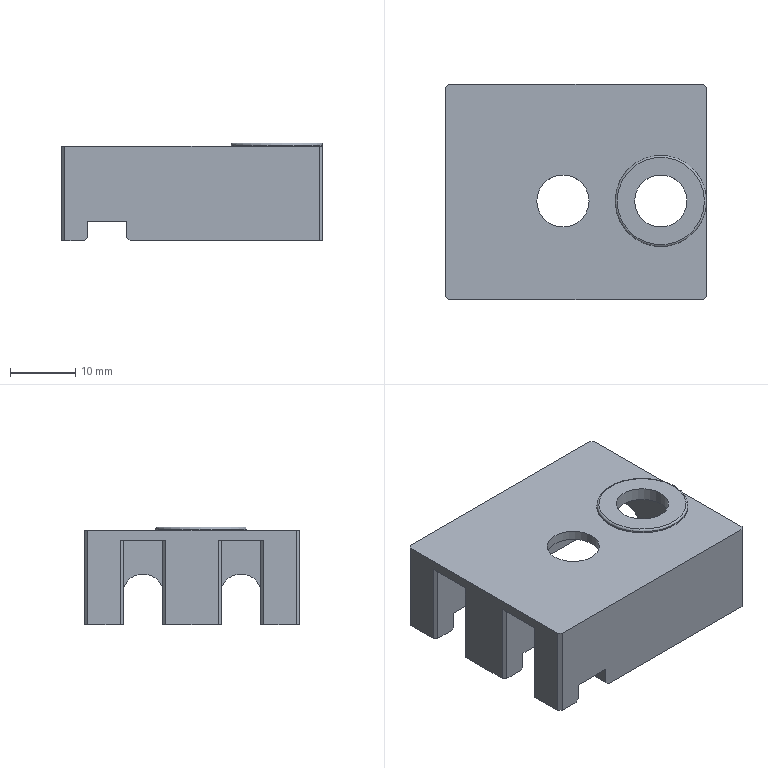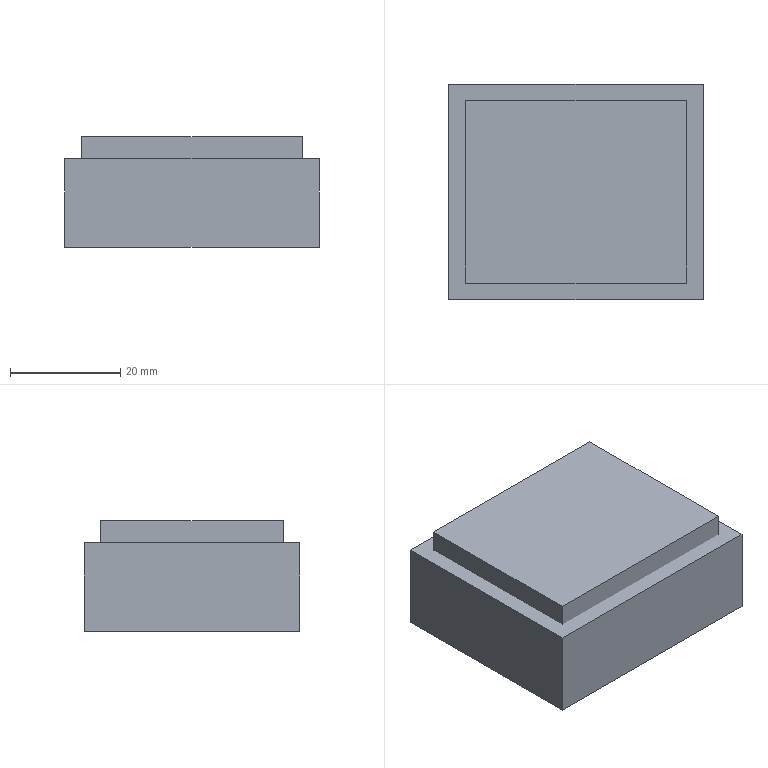CAM job | NX | 3+2 milling, drilling | part box 40 x 33 x 15 mm | stock box 46 x 39 x 20 mm
Tools:
number,name,description,diameter,corner_radius,flute_length,length,flutes
1,D63,Milling Tool-5 Parameters,63.0,0.0,50.0,75.0,2
2,D10,Milling Tool-5 Parameters,10.0,0.0,50.0,75.0,2
4,D6,Milling Tool-5 Parameters,6.0,0.0,50.0,75.0,2
9,D6A45,Milling Tool-5 Parameters,6.0,0.0,3.0,3.0,2
10,2.5ZT,Drilling Tool,2.4,0.0,35.0,50.0,2
6,D4,Milling Tool-5 Parameters,4.0,0.0,50.0,75.0,2
8,D2,Milling Tool-5 Parameters,2.0,0.0,50.0,75.0,2
19,R1.5,Milling Tool-5 Parameters,3.0,1.5,50.0,75.0,2
Operations:
program,operation,operation_type,tool,method,geometry_group,spindle_rpm,surface_speed,feed_per_tooth,feed_cut,feed_plunge,cut_length_mm,path_length_mm,cut_time_min,machine_time_min
1-45-35-20毛胚,FLOOR_WALL,VolumeBased25DMillingOperation,D63,METHOD,A,6500.0,0.0,0.0,1250.0,100.0,121.0,175.0,0.0968,0.1022
1-45-35-20毛胚,ADAPTIVE_MILLING,CavityMilling,D10,METHOD,A,7000.0,219.0,0.1429,2000.0,1000.0,897.188,981.188,0.4501,0.4585
1-45-35-20毛胚,FLOOR_WALL_1_COPY_COPY,VolumeBased25DMillingOperation,D10,METHOD,A,7000.0,219.0,0.0714,1000.0,1000.0,511.66,703.384,0.5117,0.5384
1-45-35-20毛胚,HOLE_MILLING,CylinderMilling,D6,METHOD,A,7000.0,131.0,0.1214,1700.0,100.0,80.741,219.241,0.0475,0.0613
1-45-35-20毛胚,ZLEVEL_PROFILE_1_1,ZLevelMilling,D6,METHOD,A,7000.0,131.0,0.1786,2500.0,1000.0,568,625.314,0.2291,0.2348
1-45-35-20毛胚,ZLEVEL_PROFILE_COPY_1_COPY_COPY_COPY_COPY,ZLevelMilling,D6A45,METHOD,A,7000.0,131.0,0.0714,1000.0,1000.0,197.26,419.585,0.1973,0.2195
1-45-35-20毛胚,刀补2,ZLevelMilling,D10,METHOD,A,6500.0,326.0,0.0769,1000.0,1000.0,185.444,272.444,0.1854,0.1941
1-45-35-20毛胚,刀补4,CylinderMilling,D6,METHOD,A,7000.0,131.0,0.0714,1000.0,100.0,33.73,172.23,0.0337,0.0476
2-45-35-20毛胚,FLOOR_WALL_COPY,VolumeBased25DMillingOperation,D63,METHOD,B,6500.0,0.0,0.0,1250.0,100.0,575.0,1261.001,0.46,0.5286
2-45-35-20毛胚,DRILLING,Operation,D6A45,METHOD,B,4000.0,75.0,0.0312,250.0,0.0,13.8,121.259,0.0552,0.0659
2-45-35-20毛胚,DRILLING_COPY,Operation,2.5ZT,METHOD,B,2000.0,15.0,0.025,100.0,0.0,44.13,181.918,0.4413,0.4551
2-45-35-20毛胚,CAVITY_MILL,CavityMilling,D10,METHOD,B,7000.0,219.0,0.1571,2200.0,1000.0,2692.01,3734.1,1.663,1.768
2-45-35-20毛胚,CAVITY_MILL_COPY,CavityMilling,D4,METHOD,B,7000.0,87.0,0.0857,1200.0,1000.0,5395.78,7350.997,4.607,4.803
2-45-35-20毛胚,FLOOR_WALL_1_COPY_COPY_1_COPY,VolumeBased25DMillingOperation,D4,METHOD,B,7000.0,219.0,0.0714,1000.0,1000.0,341.727,452.312,0.3417,0.3534
2-45-35-20毛胚,FLOOR_WALL_1_COPY_COPY_1,VolumeBased25DMillingOperation,D4,METHOD,B,7000.0,219.0,0.0714,1000.0,1000.0,837.288,1794.605,0.8373,0.9338
2-45-35-20毛胚,ZLEVEL_PROFILE_COPY_COPY_1_COPY,ZLevelMilling,D4,METHOD,B,6500.0,326.0,0.0769,1000.0,1000.0,44.85,356.415,0.0448,0.076
2-45-35-20毛胚,CAVITY_MILL_COPY_COPY,CavityMilling,D2,METHOD,B,7000.0,43.0,0.0714,1000.0,1000.0,1832.263,3557.423,1.832,2.005
2-45-35-20毛胚,FIXED_CONTOUR,SurfaceContour,R1.5,METHOD,B,7000.0,65.0,0.1429,2000.0,1000.0,217.85,337.954,0.1184,0.1304
2-45-35-20毛胚,ZLEVEL_PROFILE_COPY_1_COPY_COPY_COPY_COPY_COPY,ZLevelMilling,D6A45,METHOD,B,7000.0,131.0,0.0714,1000.0,1000.0,270.555,808.358,0.2706,0.3243
2-45-35-20毛胚,ZLEVEL_PROFILE_COPY_1_COPY_COPY_COPY_COPY_COPY_COPY,ZLevelMilling,D6A45,METHOD,B,7000.0,131.0,0.0714,1000.0,1000.0,35.354,260.839,0.0354,0.0579